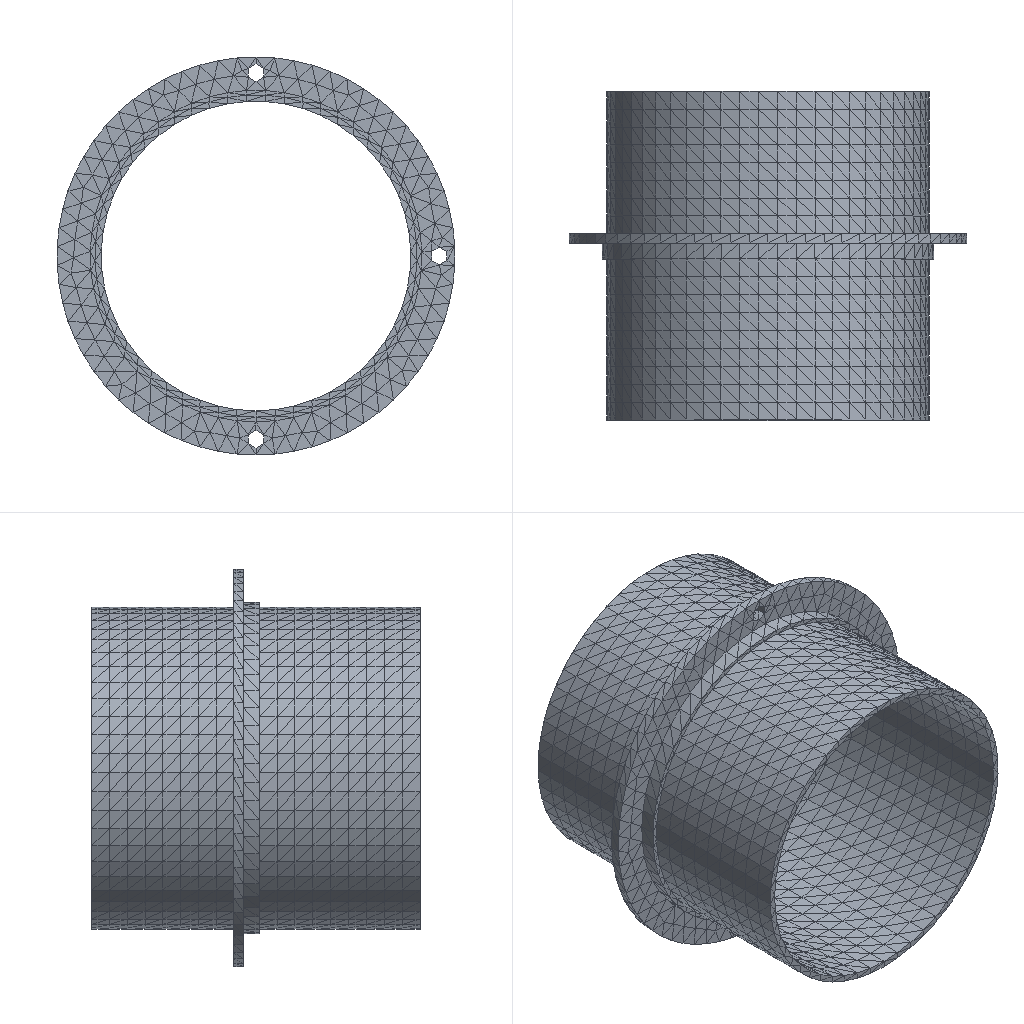Simulation study | nx simcenter
Set-up summary:
category,name,step,type,value,unit,region
solver,nx_nastran (Simcenter)
units,not stated in the deck,,not stated
analysis,deck,,static,static
analysis,solution,,SOL,101
load_step,SUBCASE 1,1,SUBCASE,SPC=1 LOAD=2
load_step,requested,,,1
mesh,nodes,,,14212
mesh,elements,,,7029
element_type,CTETRA,,solid,7029
load,nodal force total,,FX,-3500000.0,model units
load,nodal force total,,FY,0.0,model units
load,nodal force total,,FZ,0.0,model units
load,load commands in deck,,count,1325
bc,support commands in deck,,count,690
analysis,NX solution 0,,Structural,Linear Statics - Single Constraint
check,setup vs results,,match,every grid point's frame and coordinates and every element id; grid points of CTETRA elements
Nastran input file, long lists of numbers shortened:
$*$$$$$$$$$$$$$$$$$$$$$$$$$$$$$$$$$$$$$$$$$$$$$$$$$$$$$$$$$$$$$$$$$
$*
$*                    NX v10.0.0.24 TRANSLATOR
$*                    FOR NX NASTRAN VERSION 10.0
$ (33 more lines like these left out)
ASSIGN OUTPUT2='162_sim1-solution_1.op2' UNIT=12
$*
$*$$$$$$$$$$$$$$$$$$$$$$$$$$$$$$$$$$$
$*
$* EXECUTIVE CONTROL
$*
$*$$$$$$$$$$$$$$$$$$$$$$$$$$$$$$$$$$$
$*
ID,NASTRAN,162_sim1-solution_1
SOL 101
CEND
$*
$*$$$$$$$$$$$$$$$$$$$$$$$$$$$$$$$$$$$
$*
$* CASE CONTROL
$*
$*$$$$$$$$$$$$$$$$$$$$$$$$$$$$$$$$$$$
$*
TITLE = Solution 1
ECHO = NONE
SPC = 1
OUTPUT
BCRESULTS(TRACTION,FORCE,PLOT) = ALL
DISPLACEMENT(PLOT) = ALL
ESE(PLOT) = ALL
FORCE(PLOT,CORNER) = ALL
OLOAD(PLOT) = ALL
SPCFORCES(PLOT) = ALL
STRAIN(PLOT,FIBER,CORNER) = ALL
STRESS(PLOT,CORNER) = ALL
$*  NX Step: Subcase - Static Loads 1
SUBCASE 1
LABEL = Subcase - Static Loads 1
LOAD = 2
$*
$*$$$$$$$$$$$$$$$$$$$$$$$$$$$$$$$$$$$
$*
$* BULK DATA
$*
$*$$$$$$$$$$$$$$$$$$$$$$$$$$$$$$$$$$$
$*
BEGIN BULK
$*
$* PARAM CARDS
$*
PARAM      K6ROT100.0000
PARAM     OIBULK     YES
PARAM    OMACHPR     YES
PARAM       POST      -2
PARAM    POSTEXT     YES
PARAM    UNITSYS   MN-MM
$*
$* GRID CARDS
$*
GRID*              14197               00.0000000000E+00-8.200000000E+01+
*       -4.900000000E+01               0
GRID*              14198               00.0000000000E+00-8.200000000E+01+
*       -5.100000000E+01               0
$ (28420 more lines like these left out)
$*
$* ELEMENT CARDS
$*
$*  NX Mesh Collector: Solid(1)
$*  NX Mesh: 3d_mesh(1)
CTETRA         1       1   11712   13925   13924    8075      69   13954+
+             70      71   10429   10430
CTETRA         2       1   10912   14164   13762   13526   11039   10988+
+          11035      72      73   10798
$ (14054 more lines like these left out)
$*
$* PROPERTY CARDS
$*
$*  NX Property: PSOLID1
PSOLID         1       1       0                           SMECH
$*
$* MATERIAL CARDS
$*
$*  NX Material: 45
MAT1           12.1000+8        0.3100007.8500-61.7280-5
$*
$* LOAD AND CONSTRAINT CARDS
$*
$*  NX Load and Constraint: Fixed(1)
SPC            1    5023  123456  0.0000
SPC            1    5024  123456  0.0000
SPC            1    5025  123456  0.0000
SPC            1    5026  123456  0.0000
$ (686 more lines like these left out)
$*  NX Load and Constraint: Force(1)
FORCE          2   11715       0 2751.56-1.00000  0.0000  0.0000
FORCE          2   11716       0 2751.57-1.00000  0.0000  0.0000
FORCE          2   11717       0 2751.56-1.00000  0.0000  0.0000
FORCE          2   11718       0 2751.56-1.00000  0.0000  0.0000
$ (1321 more lines like these left out)
ENDDATA 8caf94c4
Results summary:
result,analysis,,,static
result,last_loadstep,,,1
result,primary field,,,displacements
result,max displacement,,,0.005242,model units
result,reaction total,,FX,3499998.75,model units
result,reaction total,,FY,0.1478,model units
result,reaction total,,FZ,-0.0372,model units
result,NX solution 0,,loadcases,1,mm